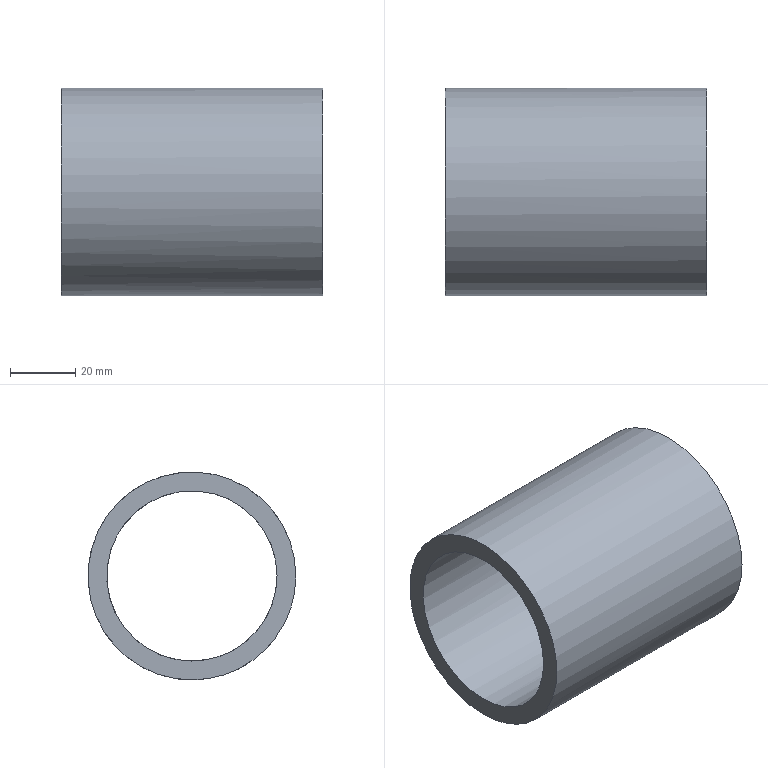Part | NX | features solid 2 | 1 solid | 4 faces | box 80 x 63.5 x 63.5 mm | volume 83456 mm3 | cylinder 2 | plane 2 | commonest cylinder face diameters 52 x1 63.5 x1
STEP:
#1=CARTESIAN_POINT('',(1205.,620.,214.));
#2=VERTEX_POINT('',#1);
#3=CARTESIAN_POINT('',(1205.,620.,240.));
#4=DIRECTION('',(1.,0.,0.));
#5=DIRECTION('',(0.,0.,-1.));
#6=AXIS2_PLACEMENT_3D('',#3,#4,#5);
#7=CIRCLE('',#6,26.);
#8=EDGE_CURVE('',#2,#2,#7,.T.);
#9=ORIENTED_EDGE('',*,*,#8,.F.);
#10=EDGE_LOOP('',(#9));
#11=FACE_BOUND('',#10,.T.);
#12=CARTESIAN_POINT('',(1285.,594.,240.));
#13=VERTEX_POINT('',#12);
#14=CARTESIAN_POINT('',(1285.,620.,240.));
#15=DIRECTION('',(1.,0.,0.));
#16=DIRECTION('',(0.,-1.,0.));
#17=AXIS2_PLACEMENT_3D('',#14,#15,#16);
#18=CIRCLE('',#17,26.);
#19=EDGE_CURVE('',#13,#13,#18,.T.);
#20=ORIENTED_EDGE('',*,*,#19,.T.);
#21=EDGE_LOOP('',(#20));
#22=FACE_BOUND('',#21,.T.);
#23=CARTESIAN_POINT('',(1225.,620.,240.));
#24=DIRECTION('',(1.,0.,0.));
#25=DIRECTION('',(0.,0.,1.));
#26=AXIS2_PLACEMENT_3D('',#23,#24,#25);
#27=CYLINDRICAL_SURFACE('',#26,26.);
#28=ADVANCED_FACE('',(#11,#22),#27,.F.);
#29=CARTESIAN_POINT('',(1205.,620.,208.25));
#30=VERTEX_POINT('',#29);
#31=CARTESIAN_POINT('',(1205.,620.,240.));
#32=DIRECTION('',(1.,0.,0.));
#33=DIRECTION('',(0.,0.,-1.));
#34=AXIS2_PLACEMENT_3D('',#31,#32,#33);
#35=CIRCLE('',#34,31.75);
#36=EDGE_CURVE('',#30,#30,#35,.T.);
#37=ORIENTED_EDGE('',*,*,#36,.T.);
#38=EDGE_LOOP('',(#37));
#39=FACE_BOUND('',#38,.T.);
#40=CARTESIAN_POINT('',(1285.,588.25,240.));
#41=VERTEX_POINT('',#40);
#42=CARTESIAN_POINT('',(1285.,620.,240.));
#43=DIRECTION('',(1.,0.,0.));
#44=DIRECTION('',(0.,-1.,0.));
#45=AXIS2_PLACEMENT_3D('',#42,#43,#44);
#46=CIRCLE('',#45,31.75);
#47=EDGE_CURVE('',#41,#41,#46,.T.);
#48=ORIENTED_EDGE('',*,*,#47,.F.);
#49=EDGE_LOOP('',(#48));
#50=FACE_BOUND('',#49,.T.);
#51=CARTESIAN_POINT('',(1225.,620.,240.));
#52=DIRECTION('',(1.,0.,0.));
#53=DIRECTION('',(0.,0.,1.));
#54=AXIS2_PLACEMENT_3D('',#51,#52,#53);
#55=CYLINDRICAL_SURFACE('',#54,31.75);
#56=ADVANCED_FACE('',(#39,#50),#55,.T.);
#57=ORIENTED_EDGE('',*,*,#8,.T.);
#58=EDGE_LOOP('',(#57));
#59=FACE_BOUND('',#58,.T.);
#60=ORIENTED_EDGE('',*,*,#36,.F.);
#61=EDGE_LOOP('',(#60));
#62=FACE_BOUND('',#61,.T.);
#63=CARTESIAN_POINT('',(1205.,550.,230.));
#64=DIRECTION('',(1.,0.,0.));
#65=DIRECTION('',(0.,0.,1.));
#66=AXIS2_PLACEMENT_3D('',#63,#64,#65);
#67=PLANE('',#66);
#68=ADVANCED_FACE('',(#59,#62),#67,.F.);
#69=ORIENTED_EDGE('',*,*,#19,.F.);
#70=EDGE_LOOP('',(#69));
#71=FACE_BOUND('',#70,.T.);
#72=ORIENTED_EDGE('',*,*,#47,.T.);
#73=EDGE_LOOP('',(#72));
#74=FACE_BOUND('',#73,.T.);
#75=CARTESIAN_POINT('',(1285.,620.,240.));
#76=DIRECTION('',(1.,0.,0.));
#77=DIRECTION('',(0.,0.,1.));
#78=AXIS2_PLACEMENT_3D('',#75,#76,#77);
#79=PLANE('',#78);
#80=ADVANCED_FACE('',(#71,#74),#79,.T.);
#81=CLOSED_SHELL('',(#28,#56,#68,#80));
#82=MANIFOLD_SOLID_BREP('',#81);
#83=(LENGTH_UNIT()NAMED_UNIT(*)SI_UNIT(.MILLI.,.METRE.));
#84=UNCERTAINTY_MEASURE_WITH_UNIT(LENGTH_MEASURE(0.00001),#83,'','');
#85=(NAMED_UNIT(*)PLANE_ANGLE_UNIT()SI_UNIT($,.RADIAN.));
#86=(NAMED_UNIT(*)SI_UNIT($,.STERADIAN.)SOLID_ANGLE_UNIT());
#87=(GEOMETRIC_REPRESENTATION_CONTEXT(3)GLOBAL_UNCERTAINTY_ASSIGNED_CONTEXT((#84))GLOBAL_UNIT_ASSIGNED_CONTEXT((#83,#85,#86))REPRESENTATION_CONTEXT('',''));
#88=ADVANCED_BREP_SHAPE_REPRESENTATION('',(#82),#87);